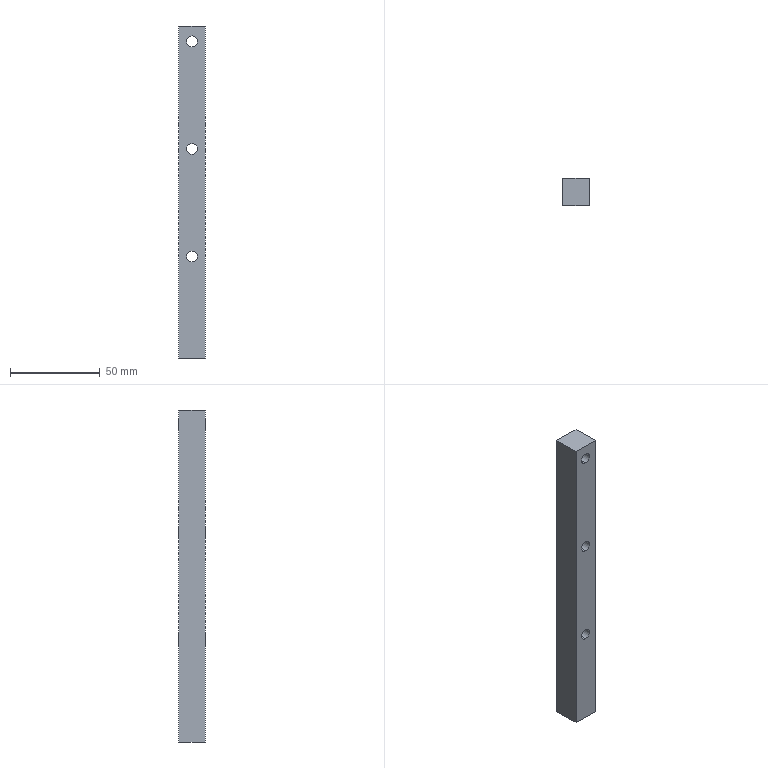Part | 1 solid | 16 faces | box 15 x 15 x 185 mm | volume 39520 mm3 | cylinder 8 | plane 6 | cone 2 | commonest cylinder face diameters 6 x6 6.8 x2
STEP:
#1=CARTESIAN_POINT('',(7.5,0.,456.));
#2=VERTEX_POINT('',#1);
#3=CARTESIAN_POINT('',(7.5,0.,462.));
#4=VERTEX_POINT('',#3);
#5=CARTESIAN_POINT('',(7.5,0.,459.));
#6=DIRECTION('',(0.,1.,0.));
#7=DIRECTION('',(0.,0.,1.));
#8=AXIS2_PLACEMENT_3D('',#5,#6,#7);
#9=CIRCLE('',#8,3.);
#10=EDGE_CURVE('',#2,#4,#9,.T.);
#11=ORIENTED_EDGE('',*,*,#10,.F.);
#12=CARTESIAN_POINT('',(7.5,15.,456.));
#13=VERTEX_POINT('',#12);
#14=CARTESIAN_POINT('',(7.5,15.,456.));
#15=DIRECTION('',(0.,1.,0.));
#16=VECTOR('',#15,1000.);
#17=LINE('',#14,#16);
#18=EDGE_CURVE('',#2,#13,#17,.T.);
#19=ORIENTED_EDGE('',*,*,#18,.T.);
#20=CARTESIAN_POINT('',(7.5,15.,462.));
#21=VERTEX_POINT('',#20);
#22=CARTESIAN_POINT('',(7.5,15.,459.));
#23=DIRECTION('',(0.,1.,0.));
#24=DIRECTION('',(0.,0.,1.));
#25=AXIS2_PLACEMENT_3D('',#22,#23,#24);
#26=CIRCLE('',#25,3.);
#27=EDGE_CURVE('',#13,#21,#26,.T.);
#28=ORIENTED_EDGE('',*,*,#27,.T.);
#29=CARTESIAN_POINT('',(7.5,15.,462.));
#30=DIRECTION('',(0.,1.,0.));
#31=VECTOR('',#30,1000.);
#32=LINE('',#29,#31);
#33=EDGE_CURVE('',#4,#21,#32,.T.);
#34=ORIENTED_EDGE('',*,*,#33,.F.);
#35=EDGE_LOOP('',(#11,#19,#28,#34));
#36=FACE_OUTER_BOUND('',#35,.T.);
#37=CARTESIAN_POINT('',(7.5,15.,459.));
#38=DIRECTION('',(0.,1.,0.));
#39=DIRECTION('',(0.,0.,1.));
#40=AXIS2_PLACEMENT_3D('',#37,#38,#39);
#41=CYLINDRICAL_SURFACE('',#40,3.);
#42=ADVANCED_FACE('',(#36),#41,.F.);
#43=CARTESIAN_POINT('',(7.5,0.,396.));
#44=VERTEX_POINT('',#43);
#45=CARTESIAN_POINT('',(7.5,0.,402.));
#46=VERTEX_POINT('',#45);
#47=CARTESIAN_POINT('',(7.5,0.,399.));
#48=DIRECTION('',(0.,1.,0.));
#49=DIRECTION('',(0.,0.,1.));
#50=AXIS2_PLACEMENT_3D('',#47,#48,#49);
#51=CIRCLE('',#50,3.);
#52=EDGE_CURVE('',#44,#46,#51,.T.);
#53=ORIENTED_EDGE('',*,*,#52,.F.);
#54=CARTESIAN_POINT('',(7.5,15.,396.));
#55=VERTEX_POINT('',#54);
#56=CARTESIAN_POINT('',(7.5,15.,396.));
#57=DIRECTION('',(0.,1.,0.));
#58=VECTOR('',#57,1000.);
#59=LINE('',#56,#58);
#60=EDGE_CURVE('',#44,#55,#59,.T.);
#61=ORIENTED_EDGE('',*,*,#60,.T.);
#62=CARTESIAN_POINT('',(7.5,15.,402.));
#63=VERTEX_POINT('',#62);
#64=CARTESIAN_POINT('',(7.5,15.,399.));
#65=DIRECTION('',(0.,1.,0.));
#66=DIRECTION('',(0.,0.,1.));
#67=AXIS2_PLACEMENT_3D('',#64,#65,#66);
#68=CIRCLE('',#67,3.);
#69=EDGE_CURVE('',#55,#63,#68,.T.);
#70=ORIENTED_EDGE('',*,*,#69,.T.);
#71=CARTESIAN_POINT('',(7.5,15.,402.));
#72=DIRECTION('',(0.,1.,0.));
#73=VECTOR('',#72,1000.);
#74=LINE('',#71,#73);
#75=EDGE_CURVE('',#46,#63,#74,.T.);
#76=ORIENTED_EDGE('',*,*,#75,.F.);
#77=EDGE_LOOP('',(#53,#61,#70,#76));
#78=FACE_OUTER_BOUND('',#77,.T.);
#79=CARTESIAN_POINT('',(7.5,15.,399.));
#80=DIRECTION('',(0.,1.,0.));
#81=DIRECTION('',(0.,0.,1.));
#82=AXIS2_PLACEMENT_3D('',#79,#80,#81);
#83=CYLINDRICAL_SURFACE('',#82,3.);
#84=ADVANCED_FACE('',(#78),#83,.F.);
#85=CARTESIAN_POINT('',(7.5,0.,336.));
#86=VERTEX_POINT('',#85);
#87=CARTESIAN_POINT('',(7.5,0.,342.));
#88=VERTEX_POINT('',#87);
#89=CARTESIAN_POINT('',(7.5,0.,339.));
#90=DIRECTION('',(0.,1.,0.));
#91=DIRECTION('',(0.,0.,1.));
#92=AXIS2_PLACEMENT_3D('',#89,#90,#91);
#93=CIRCLE('',#92,3.);
#94=EDGE_CURVE('',#86,#88,#93,.T.);
#95=ORIENTED_EDGE('',*,*,#94,.F.);
#96=CARTESIAN_POINT('',(7.5,15.,336.));
#97=VERTEX_POINT('',#96);
#98=CARTESIAN_POINT('',(7.5,15.,336.));
#99=DIRECTION('',(0.,1.,0.));
#100=VECTOR('',#99,1000.);
#101=LINE('',#98,#100);
#102=EDGE_CURVE('',#86,#97,#101,.T.);
#103=ORIENTED_EDGE('',*,*,#102,.T.);
#104=CARTESIAN_POINT('',(7.5,15.,342.));
#105=VERTEX_POINT('',#104);
#106=CARTESIAN_POINT('',(7.5,15.,339.));
#107=DIRECTION('',(0.,1.,0.));
#108=DIRECTION('',(0.,0.,1.));
#109=AXIS2_PLACEMENT_3D('',#106,#107,#108);
#110=CIRCLE('',#109,3.);
#111=EDGE_CURVE('',#97,#105,#110,.T.);
#112=ORIENTED_EDGE('',*,*,#111,.T.);
#113=CARTESIAN_POINT('',(7.5,15.,342.));
#114=DIRECTION('',(0.,1.,0.));
#115=VECTOR('',#114,1000.);
#116=LINE('',#113,#115);
#117=EDGE_CURVE('',#88,#105,#116,.T.);
#118=ORIENTED_EDGE('',*,*,#117,.F.);
#119=EDGE_LOOP('',(#95,#103,#112,#118));
#120=FACE_OUTER_BOUND('',#119,.T.);
#121=CARTESIAN_POINT('',(7.5,15.,339.));
#122=DIRECTION('',(0.,1.,0.));
#123=DIRECTION('',(0.,0.,1.));
#124=AXIS2_PLACEMENT_3D('',#121,#122,#123);
#125=CYLINDRICAL_SURFACE('',#124,3.);
#126=ADVANCED_FACE('',(#120),#125,.F.);
#127=CARTESIAN_POINT('',(10.9,7.5,304.75));
#128=VERTEX_POINT('',#127);
#129=CARTESIAN_POINT('',(4.1,7.5,304.75));
#130=VERTEX_POINT('',#129);
#131=CARTESIAN_POINT('',(7.5,7.5,304.75));
#132=DIRECTION('',(0.,0.,-1.));
#133=DIRECTION('',(-1.,0.,0.));
#134=AXIS2_PLACEMENT_3D('',#131,#132,#133);
#135=CIRCLE('',#134,3.4);
#136=EDGE_CURVE('',#128,#130,#135,.T.);
#137=ORIENTED_EDGE('',*,*,#136,.F.);
#138=CARTESIAN_POINT('',(10.9,7.5,282.5));
#139=VERTEX_POINT('',#138);
#140=CARTESIAN_POINT('',(10.9,7.5,282.5));
#141=DIRECTION('',(0.,0.,-1.));
#142=VECTOR('',#141,1000.);
#143=LINE('',#140,#142);
#144=EDGE_CURVE('',#128,#139,#143,.T.);
#145=ORIENTED_EDGE('',*,*,#144,.T.);
#146=CARTESIAN_POINT('',(4.1,7.5,282.5));
#147=VERTEX_POINT('',#146);
#148=CARTESIAN_POINT('',(7.5,7.5,282.5));
#149=DIRECTION('',(0.,0.,-1.));
#150=DIRECTION('',(-1.,0.,0.));
#151=AXIS2_PLACEMENT_3D('',#148,#149,#150);
#152=CIRCLE('',#151,3.4);
#153=EDGE_CURVE('',#139,#147,#152,.T.);
#154=ORIENTED_EDGE('',*,*,#153,.T.);
#155=CARTESIAN_POINT('',(4.1,7.5,282.5));
#156=DIRECTION('',(0.,0.,-1.));
#157=VECTOR('',#156,1000.);
#158=LINE('',#155,#157);
#159=EDGE_CURVE('',#130,#147,#158,.T.);
#160=ORIENTED_EDGE('',*,*,#159,.F.);
#161=EDGE_LOOP('',(#137,#145,#154,#160));
#162=FACE_OUTER_BOUND('',#161,.T.);
#163=CARTESIAN_POINT('',(7.5,7.5,282.5));
#164=DIRECTION('',(0.,0.,-1.));
#165=DIRECTION('',(-1.,0.,0.));
#166=AXIS2_PLACEMENT_3D('',#163,#164,#165);
#167=CYLINDRICAL_SURFACE('',#166,3.4);
#168=ADVANCED_FACE('',(#162),#167,.F.);
#169=CARTESIAN_POINT('',(7.5,7.5,306.793));
#170=VERTEX_POINT('',#169);
#171=CARTESIAN_POINT('',(4.1,7.5,304.75));
#172=DIRECTION('',(-0.8572,0.,-0.515));
#173=VECTOR('',#172,1000.);
#174=LINE('',#171,#173);
#175=EDGE_CURVE('',#170,#130,#174,.T.);
#176=ORIENTED_EDGE('',*,*,#175,.F.);
#177=CARTESIAN_POINT('',(10.9,7.5,304.75));
#178=DIRECTION('',(0.8572,0.,-0.515));
#179=VECTOR('',#178,1000.);
#180=LINE('',#177,#179);
#181=EDGE_CURVE('',#170,#128,#180,.T.);
#182=ORIENTED_EDGE('',*,*,#181,.T.);
#183=ORIENTED_EDGE('',*,*,#136,.T.);
#184=EDGE_LOOP('',(#176,#182,#183));
#185=FACE_OUTER_BOUND('',#184,.T.);
#186=CARTESIAN_POINT('',(7.5,7.5,304.75));
#187=DIRECTION('',(0.,0.,-1.));
#188=DIRECTION('',(-1.,0.,0.));
#189=AXIS2_PLACEMENT_3D('',#186,#187,#188);
#190=CONICAL_SURFACE('',#189,3.4,1.03);
#191=ADVANCED_FACE('',(#185),#190,.F.);
#192=CARTESIAN_POINT('',(7.5,15.,459.));
#193=DIRECTION('',(0.,1.,0.));
#194=DIRECTION('',(0.,0.,1.));
#195=AXIS2_PLACEMENT_3D('',#192,#193,#194);
#196=CIRCLE('',#195,3.);
#197=EDGE_CURVE('',#21,#13,#196,.T.);
#198=ORIENTED_EDGE('',*,*,#197,.F.);
#199=ORIENTED_EDGE('',*,*,#27,.F.);
#200=EDGE_LOOP('',(#198,#199));
#201=FACE_BOUND('',#200,.T.);
#202=CARTESIAN_POINT('',(7.5,15.,399.));
#203=DIRECTION('',(0.,1.,0.));
#204=DIRECTION('',(0.,0.,1.));
#205=AXIS2_PLACEMENT_3D('',#202,#203,#204);
#206=CIRCLE('',#205,3.);
#207=EDGE_CURVE('',#63,#55,#206,.T.);
#208=ORIENTED_EDGE('',*,*,#207,.F.);
#209=ORIENTED_EDGE('',*,*,#69,.F.);
#210=EDGE_LOOP('',(#208,#209));
#211=FACE_BOUND('',#210,.T.);
#212=CARTESIAN_POINT('',(15.,15.,467.5));
#213=VERTEX_POINT('',#212);
#214=CARTESIAN_POINT('',(15.,15.,282.5));
#215=VERTEX_POINT('',#214);
#216=CARTESIAN_POINT('',(15.,15.,720.));
#217=DIRECTION('',(0.,0.,-1.));
#218=VECTOR('',#217,1000.);
#219=LINE('',#216,#218);
#220=EDGE_CURVE('',#213,#215,#219,.T.);
#221=ORIENTED_EDGE('',*,*,#220,.T.);
#222=CARTESIAN_POINT('',(0.,15.,282.5));
#223=VERTEX_POINT('',#222);
#224=CARTESIAN_POINT('',(0.,15.,282.5));
#225=DIRECTION('',(1.,0.,0.));
#226=VECTOR('',#225,1000.);
#227=LINE('',#224,#226);
#228=EDGE_CURVE('',#223,#215,#227,.T.);
#229=ORIENTED_EDGE('',*,*,#228,.F.);
#230=CARTESIAN_POINT('',(0.,15.,467.5));
#231=VERTEX_POINT('',#230);
#232=CARTESIAN_POINT('',(0.,15.,720.));
#233=DIRECTION('',(0.,0.,-1.));
#234=VECTOR('',#233,1000.);
#235=LINE('',#232,#234);
#236=EDGE_CURVE('',#231,#223,#235,.T.);
#237=ORIENTED_EDGE('',*,*,#236,.F.);
#238=CARTESIAN_POINT('',(0.,15.,467.5));
#239=DIRECTION('',(-1.,0.,0.));
#240=VECTOR('',#239,1000.);
#241=LINE('',#238,#240);
#242=EDGE_CURVE('',#213,#231,#241,.T.);
#243=ORIENTED_EDGE('',*,*,#242,.F.);
#244=EDGE_LOOP('',(#221,#229,#237,#243));
#245=FACE_OUTER_BOUND('',#244,.T.);
#246=CARTESIAN_POINT('',(7.5,15.,339.));
#247=DIRECTION('',(0.,1.,0.));
#248=DIRECTION('',(0.,0.,1.));
#249=AXIS2_PLACEMENT_3D('',#246,#247,#248);
#250=CIRCLE('',#249,3.);
#251=EDGE_CURVE('',#105,#97,#250,.T.);
#252=ORIENTED_EDGE('',*,*,#251,.F.);
#253=ORIENTED_EDGE('',*,*,#111,.F.);
#254=EDGE_LOOP('',(#252,#253));
#255=FACE_BOUND('',#254,.T.);
#256=CARTESIAN_POINT('',(0.,15.,720.));
#257=DIRECTION('',(0.,-1.,0.));
#258=DIRECTION('',(0.,0.,-1.));
#259=AXIS2_PLACEMENT_3D('',#256,#257,#258);
#260=PLANE('',#259);
#261=ADVANCED_FACE('',(#201,#211,#245,#255),#260,.F.);
#262=ORIENTED_EDGE('',*,*,#236,.T.);
#263=CARTESIAN_POINT('',(0.,0.,282.5));
#264=VERTEX_POINT('',#263);
#265=CARTESIAN_POINT('',(0.,0.,282.5));
#266=DIRECTION('',(0.,1.,0.));
#267=VECTOR('',#266,1000.);
#268=LINE('',#265,#267);
#269=EDGE_CURVE('',#264,#223,#268,.T.);
#270=ORIENTED_EDGE('',*,*,#269,.F.);
#271=CARTESIAN_POINT('',(0.,0.,467.5));
#272=VERTEX_POINT('',#271);
#273=CARTESIAN_POINT('',(0.,0.,720.));
#274=DIRECTION('',(0.,0.,-1.));
#275=VECTOR('',#274,1000.);
#276=LINE('',#273,#275);
#277=EDGE_CURVE('',#272,#264,#276,.T.);
#278=ORIENTED_EDGE('',*,*,#277,.F.);
#279=CARTESIAN_POINT('',(0.,0.,467.5));
#280=DIRECTION('',(0.,1.,0.));
#281=VECTOR('',#280,1000.);
#282=LINE('',#279,#281);
#283=EDGE_CURVE('',#272,#231,#282,.T.);
#284=ORIENTED_EDGE('',*,*,#283,.T.);
#285=EDGE_LOOP('',(#262,#270,#278,#284));
#286=FACE_OUTER_BOUND('',#285,.T.);
#287=CARTESIAN_POINT('',(0.,0.,720.));
#288=DIRECTION('',(1.,0.,0.));
#289=DIRECTION('',(0.,0.,-1.));
#290=AXIS2_PLACEMENT_3D('',#287,#288,#289);
#291=PLANE('',#290);
#292=ADVANCED_FACE('',(#286),#291,.F.);
#293=CARTESIAN_POINT('',(7.5,0.,459.));
#294=DIRECTION('',(0.,1.,0.));
#295=DIRECTION('',(0.,0.,1.));
#296=AXIS2_PLACEMENT_3D('',#293,#294,#295);
#297=CIRCLE('',#296,3.);
#298=EDGE_CURVE('',#4,#2,#297,.T.);
#299=ORIENTED_EDGE('',*,*,#298,.T.);
#300=ORIENTED_EDGE('',*,*,#10,.T.);
#301=EDGE_LOOP('',(#299,#300));
#302=FACE_BOUND('',#301,.T.);
#303=CARTESIAN_POINT('',(7.5,0.,399.));
#304=DIRECTION('',(0.,1.,0.));
#305=DIRECTION('',(0.,0.,1.));
#306=AXIS2_PLACEMENT_3D('',#303,#304,#305);
#307=CIRCLE('',#306,3.);
#308=EDGE_CURVE('',#46,#44,#307,.T.);
#309=ORIENTED_EDGE('',*,*,#308,.T.);
#310=ORIENTED_EDGE('',*,*,#52,.T.);
#311=EDGE_LOOP('',(#309,#310));
#312=FACE_BOUND('',#311,.T.);
#313=CARTESIAN_POINT('',(7.5,0.,339.));
#314=DIRECTION('',(0.,1.,0.));
#315=DIRECTION('',(0.,0.,1.));
#316=AXIS2_PLACEMENT_3D('',#313,#314,#315);
#317=CIRCLE('',#316,3.);
#318=EDGE_CURVE('',#88,#86,#317,.T.);
#319=ORIENTED_EDGE('',*,*,#318,.T.);
#320=ORIENTED_EDGE('',*,*,#94,.T.);
#321=EDGE_LOOP('',(#319,#320));
#322=FACE_BOUND('',#321,.T.);
#323=ORIENTED_EDGE('',*,*,#277,.T.);
#324=CARTESIAN_POINT('',(15.,0.,282.5));
#325=VERTEX_POINT('',#324);
#326=CARTESIAN_POINT('',(0.,0.,282.5));
#327=DIRECTION('',(1.,0.,0.));
#328=VECTOR('',#327,1000.);
#329=LINE('',#326,#328);
#330=EDGE_CURVE('',#264,#325,#329,.T.);
#331=ORIENTED_EDGE('',*,*,#330,.T.);
#332=CARTESIAN_POINT('',(15.,0.,467.5));
#333=VERTEX_POINT('',#332);
#334=CARTESIAN_POINT('',(15.,0.,720.));
#335=DIRECTION('',(0.,0.,-1.));
#336=VECTOR('',#335,1000.);
#337=LINE('',#334,#336);
#338=EDGE_CURVE('',#333,#325,#337,.T.);
#339=ORIENTED_EDGE('',*,*,#338,.F.);
#340=CARTESIAN_POINT('',(0.,0.,467.5));
#341=DIRECTION('',(-1.,0.,0.));
#342=VECTOR('',#341,1000.);
#343=LINE('',#340,#342);
#344=EDGE_CURVE('',#333,#272,#343,.T.);
#345=ORIENTED_EDGE('',*,*,#344,.T.);
#346=EDGE_LOOP('',(#323,#331,#339,#345));
#347=FACE_OUTER_BOUND('',#346,.T.);
#348=CARTESIAN_POINT('',(0.,0.,720.));
#349=DIRECTION('',(0.,1.,0.));
#350=DIRECTION('',(0.,0.,1.));
#351=AXIS2_PLACEMENT_3D('',#348,#349,#350);
#352=PLANE('',#351);
#353=ADVANCED_FACE('',(#302,#312,#322,#347),#352,.F.);
#354=ORIENTED_EDGE('',*,*,#338,.T.);
#355=CARTESIAN_POINT('',(15.,0.,282.5));
#356=DIRECTION('',(0.,1.,0.));
#357=VECTOR('',#356,1000.);
#358=LINE('',#355,#357);
#359=EDGE_CURVE('',#325,#215,#358,.T.);
#360=ORIENTED_EDGE('',*,*,#359,.T.);
#361=ORIENTED_EDGE('',*,*,#220,.F.);
#362=CARTESIAN_POINT('',(15.,0.,467.5));
#363=DIRECTION('',(0.,1.,0.));
#364=VECTOR('',#363,1000.);
#365=LINE('',#362,#364);
#366=EDGE_CURVE('',#333,#213,#365,.T.);
#367=ORIENTED_EDGE('',*,*,#366,.F.);
#368=EDGE_LOOP('',(#354,#360,#361,#367));
#369=FACE_OUTER_BOUND('',#368,.T.);
#370=CARTESIAN_POINT('',(15.,0.,720.));
#371=DIRECTION('',(-1.,0.,0.));
#372=DIRECTION('',(0.,0.,1.));
#373=AXIS2_PLACEMENT_3D('',#370,#371,#372);
#374=PLANE('',#373);
#375=ADVANCED_FACE('',(#369),#374,.F.);
#376=ORIENTED_EDGE('',*,*,#242,.T.);
#377=ORIENTED_EDGE('',*,*,#283,.F.);
#378=ORIENTED_EDGE('',*,*,#344,.F.);
#379=ORIENTED_EDGE('',*,*,#366,.T.);
#380=EDGE_LOOP('',(#376,#377,#378,#379));
#381=FACE_OUTER_BOUND('',#380,.T.);
#382=CARTESIAN_POINT('',(0.,0.,467.5));
#383=DIRECTION('',(0.,0.,-1.));
#384=DIRECTION('',(-1.,0.,0.));
#385=AXIS2_PLACEMENT_3D('',#382,#383,#384);
#386=PLANE('',#385);
#387=ADVANCED_FACE('',(#381),#386,.F.);
#388=CARTESIAN_POINT('',(7.5,7.5,282.5));
#389=DIRECTION('',(0.,0.,-1.));
#390=DIRECTION('',(-1.,0.,0.));
#391=AXIS2_PLACEMENT_3D('',#388,#389,#390);
#392=CIRCLE('',#391,3.4);
#393=EDGE_CURVE('',#147,#139,#392,.T.);
#394=ORIENTED_EDGE('',*,*,#393,.F.);
#395=ORIENTED_EDGE('',*,*,#153,.F.);
#396=EDGE_LOOP('',(#394,#395));
#397=FACE_BOUND('',#396,.T.);
#398=ORIENTED_EDGE('',*,*,#228,.T.);
#399=ORIENTED_EDGE('',*,*,#359,.F.);
#400=ORIENTED_EDGE('',*,*,#330,.F.);
#401=ORIENTED_EDGE('',*,*,#269,.T.);
#402=EDGE_LOOP('',(#398,#399,#400,#401));
#403=FACE_OUTER_BOUND('',#402,.T.);
#404=CARTESIAN_POINT('',(0.,0.,282.5));
#405=DIRECTION('',(0.,0.,1.));
#406=DIRECTION('',(1.,0.,0.));
#407=AXIS2_PLACEMENT_3D('',#404,#405,#406);
#408=PLANE('',#407);
#409=ADVANCED_FACE('',(#397,#403),#408,.F.);
#410=ORIENTED_EDGE('',*,*,#181,.F.);
#411=ORIENTED_EDGE('',*,*,#175,.T.);
#412=CARTESIAN_POINT('',(7.5,7.5,304.75));
#413=DIRECTION('',(0.,0.,-1.));
#414=DIRECTION('',(-1.,0.,0.));
#415=AXIS2_PLACEMENT_3D('',#412,#413,#414);
#416=CIRCLE('',#415,3.4);
#417=EDGE_CURVE('',#130,#128,#416,.T.);
#418=ORIENTED_EDGE('',*,*,#417,.T.);
#419=EDGE_LOOP('',(#410,#411,#418));
#420=FACE_OUTER_BOUND('',#419,.T.);
#421=CARTESIAN_POINT('',(7.5,7.5,304.75));
#422=DIRECTION('',(0.,0.,-1.));
#423=DIRECTION('',(-1.,0.,0.));
#424=AXIS2_PLACEMENT_3D('',#421,#422,#423);
#425=CONICAL_SURFACE('',#424,3.4,1.03);
#426=ADVANCED_FACE('',(#420),#425,.F.);
#427=ORIENTED_EDGE('',*,*,#144,.F.);
#428=ORIENTED_EDGE('',*,*,#417,.F.);
#429=ORIENTED_EDGE('',*,*,#159,.T.);
#430=ORIENTED_EDGE('',*,*,#393,.T.);
#431=EDGE_LOOP('',(#427,#428,#429,#430));
#432=FACE_OUTER_BOUND('',#431,.T.);
#433=CARTESIAN_POINT('',(7.5,7.5,282.5));
#434=DIRECTION('',(0.,0.,-1.));
#435=DIRECTION('',(-1.,0.,0.));
#436=AXIS2_PLACEMENT_3D('',#433,#434,#435);
#437=CYLINDRICAL_SURFACE('',#436,3.4);
#438=ADVANCED_FACE('',(#432),#437,.F.);
#439=ORIENTED_EDGE('',*,*,#102,.F.);
#440=ORIENTED_EDGE('',*,*,#318,.F.);
#441=ORIENTED_EDGE('',*,*,#117,.T.);
#442=ORIENTED_EDGE('',*,*,#251,.T.);
#443=EDGE_LOOP('',(#439,#440,#441,#442));
#444=FACE_OUTER_BOUND('',#443,.T.);
#445=CARTESIAN_POINT('',(7.5,15.,339.));
#446=DIRECTION('',(0.,1.,0.));
#447=DIRECTION('',(0.,0.,1.));
#448=AXIS2_PLACEMENT_3D('',#445,#446,#447);
#449=CYLINDRICAL_SURFACE('',#448,3.);
#450=ADVANCED_FACE('',(#444),#449,.F.);
#451=ORIENTED_EDGE('',*,*,#60,.F.);
#452=ORIENTED_EDGE('',*,*,#308,.F.);
#453=ORIENTED_EDGE('',*,*,#75,.T.);
#454=ORIENTED_EDGE('',*,*,#207,.T.);
#455=EDGE_LOOP('',(#451,#452,#453,#454));
#456=FACE_OUTER_BOUND('',#455,.T.);
#457=CARTESIAN_POINT('',(7.5,15.,399.));
#458=DIRECTION('',(0.,1.,0.));
#459=DIRECTION('',(0.,0.,1.));
#460=AXIS2_PLACEMENT_3D('',#457,#458,#459);
#461=CYLINDRICAL_SURFACE('',#460,3.);
#462=ADVANCED_FACE('',(#456),#461,.F.);
#463=ORIENTED_EDGE('',*,*,#18,.F.);
#464=ORIENTED_EDGE('',*,*,#298,.F.);
#465=ORIENTED_EDGE('',*,*,#33,.T.);
#466=ORIENTED_EDGE('',*,*,#197,.T.);
#467=EDGE_LOOP('',(#463,#464,#465,#466));
#468=FACE_OUTER_BOUND('',#467,.T.);
#469=CARTESIAN_POINT('',(7.5,15.,459.));
#470=DIRECTION('',(0.,1.,0.));
#471=DIRECTION('',(0.,0.,1.));
#472=AXIS2_PLACEMENT_3D('',#469,#470,#471);
#473=CYLINDRICAL_SURFACE('',#472,3.);
#474=ADVANCED_FACE('',(#468),#473,.F.);
#475=CLOSED_SHELL('',(#42,#84,#126,#168,#191,#261,#292,#353,#375,#387,#409,#426,#438,#450,#462,#474));
#476=MANIFOLD_SOLID_BREP('',#475);
#477=CARTESIAN_POINT('',(0.,0.,0.));
#478=DIRECTION('',(0.,0.,1.));
#479=DIRECTION('',(1.,0.,0.));
#480=AXIS2_PLACEMENT_3D('',#477,#478,#479);
#481=(LENGTH_UNIT()NAMED_UNIT(*)SI_UNIT(.MILLI.,.METRE.));
#482=UNCERTAINTY_MEASURE_WITH_UNIT(LENGTH_MEASURE(0.00001),#481,'','');
#483=(NAMED_UNIT(*)PLANE_ANGLE_UNIT()SI_UNIT($,.RADIAN.));
#484=(NAMED_UNIT(*)SI_UNIT($,.STERADIAN.)SOLID_ANGLE_UNIT());
#485=(GEOMETRIC_REPRESENTATION_CONTEXT(3)GLOBAL_UNCERTAINTY_ASSIGNED_CONTEXT((#482))GLOBAL_UNIT_ASSIGNED_CONTEXT((#481,#483,#484))REPRESENTATION_CONTEXT('',''));
#486=ADVANCED_BREP_SHAPE_REPRESENTATION('',(#476,#480),#485);